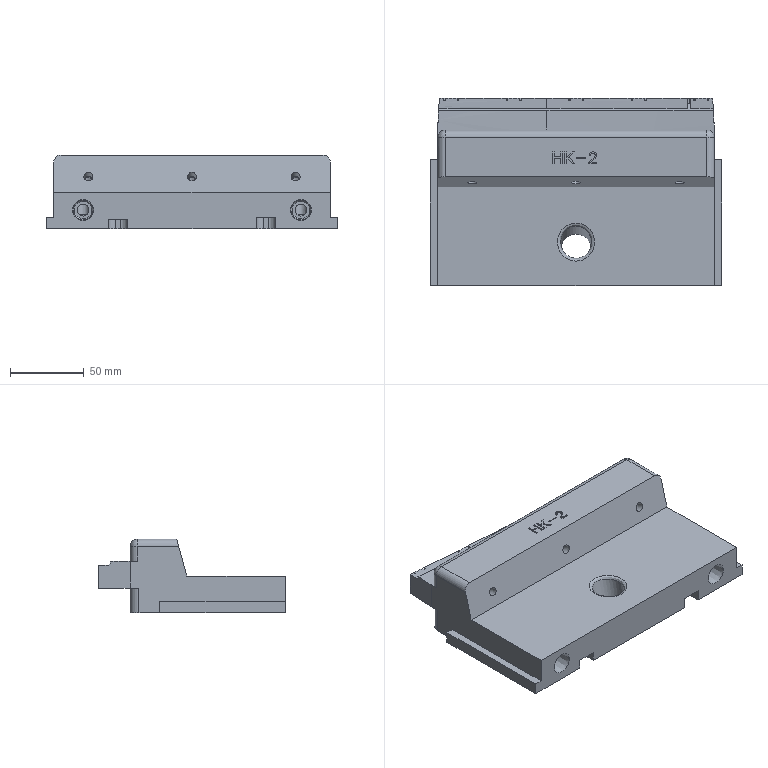Part | STEP file | solid 17 | 1 solid | 177 faces | box 197 x 126.362 x 50 mm | volume 664988 mm3 | plane 107 | cylinder 43 | cone 17 | torus 5 | sphere 2 | other 2 | spline 1 | commonest cylinder face diameters 10 x12 8 x5 4377 x5 12 x4 5 x3 6 x3